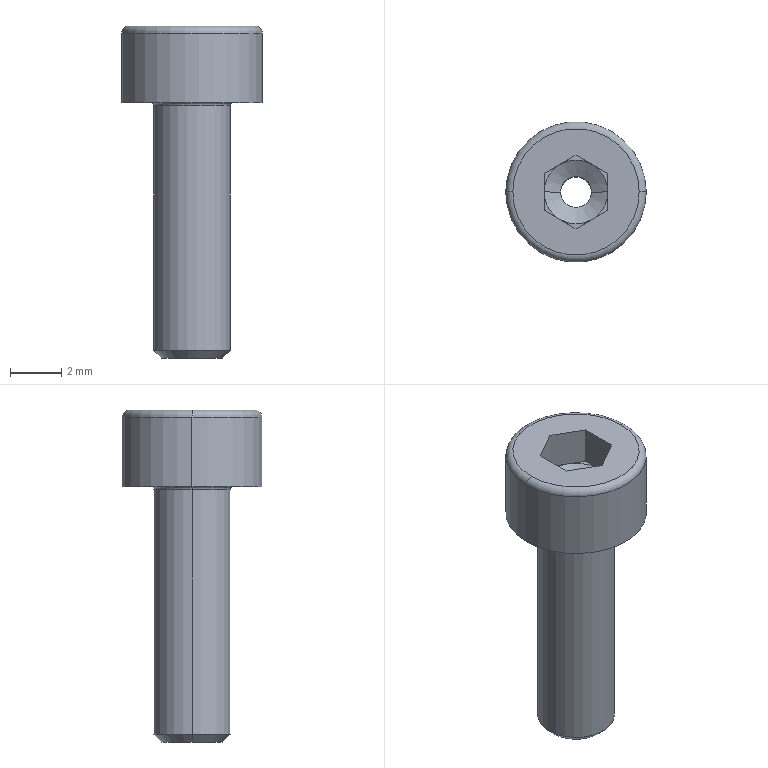Part | SolidWorks | features Fillet 2, ICE 2, Chamfer 1, Revolution 1 | 1 solid | 29 faces | box 5.5 x 5.5 x 13 mm | volume 119.572 mm3 | plane 15 | cylinder 6 | torus 4 | cone 4 | commonest cylinder face diameters 1.2 x2 3 x2 5.5 x2
STEP:
#1=CARTESIAN_POINT('',(-1.625,0.,0.));
#2=VERTEX_POINT('',#1);
#3=CARTESIAN_POINT('',(1.625,0.,0.));
#4=VERTEX_POINT('',#3);
#5=CARTESIAN_POINT('',(0.,0.,0.));
#6=DIRECTION('',(0.,0.,1.));
#7=DIRECTION('',(1.,0.,0.));
#8=AXIS2_PLACEMENT_3D('',#5,#6,#7);
#9=CIRCLE('',#8,1.625);
#10=EDGE_CURVE('',#2,#4,#9,.T.);
#11=ORIENTED_EDGE('',*,*,#10,.F.);
#12=CARTESIAN_POINT('',(-1.5,0.,-0.125));
#13=VERTEX_POINT('',#12);
#14=CARTESIAN_POINT('',(-1.625,0.,-0.125));
#15=DIRECTION('',(0.,1.,0.));
#16=DIRECTION('',(-1.,0.,0.));
#17=AXIS2_PLACEMENT_3D('',#14,#15,#16);
#18=CIRCLE('',#17,0.125);
#19=EDGE_CURVE('',#2,#13,#18,.T.);
#20=ORIENTED_EDGE('',*,*,#19,.T.);
#21=CARTESIAN_POINT('',(1.5,0.,-0.125));
#22=VERTEX_POINT('',#21);
#23=CARTESIAN_POINT('',(0.,0.,-0.125));
#24=DIRECTION('',(0.,0.,-1.));
#25=DIRECTION('',(1.,0.,0.));
#26=AXIS2_PLACEMENT_3D('',#23,#24,#25);
#27=CIRCLE('',#26,1.5);
#28=EDGE_CURVE('',#22,#13,#27,.T.);
#29=ORIENTED_EDGE('',*,*,#28,.F.);
#30=CARTESIAN_POINT('',(1.625,0.,-0.125));
#31=DIRECTION('',(0.,-1.,0.));
#32=DIRECTION('',(0.,0.,-1.));
#33=AXIS2_PLACEMENT_3D('',#30,#31,#32);
#34=CIRCLE('',#33,0.125);
#35=EDGE_CURVE('',#4,#22,#34,.T.);
#36=ORIENTED_EDGE('',*,*,#35,.F.);
#37=EDGE_LOOP('',(#11,#20,#29,#36));
#38=FACE_OUTER_BOUND('',#37,.T.);
#39=CARTESIAN_POINT('',(0.,0.,-0.125));
#40=DIRECTION('',(0.,0.,1.));
#41=DIRECTION('',(1.,0.,0.));
#42=AXIS2_PLACEMENT_3D('',#39,#40,#41);
#43=TOROIDAL_SURFACE('',#42,1.625,0.125);
#44=ADVANCED_FACE('',(#38),#43,.F.);
#45=CARTESIAN_POINT('',(-0.6,0.,1.125));
#46=VERTEX_POINT('',#45);
#47=CARTESIAN_POINT('',(0.6,0.,1.125));
#48=VERTEX_POINT('',#47);
#49=CARTESIAN_POINT('',(0.,0.,1.125));
#50=DIRECTION('',(0.,0.,1.));
#51=DIRECTION('',(1.,0.,0.));
#52=AXIS2_PLACEMENT_3D('',#49,#50,#51);
#53=CIRCLE('',#52,0.6);
#54=EDGE_CURVE('',#46,#48,#53,.T.);
#55=ORIENTED_EDGE('',*,*,#54,.F.);
#56=CARTESIAN_POINT('',(-1.25,0.,1.5));
#57=VERTEX_POINT('',#56);
#58=CARTESIAN_POINT('',(-1.25,0.,1.5));
#59=DIRECTION('',(-0.866,0.,0.5));
#60=VECTOR('',#59,1000.);
#61=LINE('',#58,#60);
#62=EDGE_CURVE('',#46,#57,#61,.T.);
#63=ORIENTED_EDGE('',*,*,#62,.T.);
#64=CARTESIAN_POINT('',(-0.625,-1.083,1.5));
#65=VERTEX_POINT('',#64);
#66=CARTESIAN_POINT('',(0.,0.,1.5));
#67=DIRECTION('',(0.,0.,1.));
#68=DIRECTION('',(1.,0.,0.));
#69=AXIS2_PLACEMENT_3D('',#66,#67,#68);
#70=CIRCLE('',#69,1.25);
#71=EDGE_CURVE('',#57,#65,#70,.T.);
#72=ORIENTED_EDGE('',*,*,#71,.T.);
#73=CARTESIAN_POINT('',(0.625,-1.083,1.5));
#74=VERTEX_POINT('',#73);
#75=CARTESIAN_POINT('',(0.,0.,1.5));
#76=DIRECTION('',(0.,0.,1.));
#77=DIRECTION('',(1.,0.,0.));
#78=AXIS2_PLACEMENT_3D('',#75,#76,#77);
#79=CIRCLE('',#78,1.25);
#80=EDGE_CURVE('',#65,#74,#79,.T.);
#81=ORIENTED_EDGE('',*,*,#80,.T.);
#82=CARTESIAN_POINT('',(1.25,0.,1.5));
#83=VERTEX_POINT('',#82);
#84=CARTESIAN_POINT('',(0.,0.,1.5));
#85=DIRECTION('',(0.,0.,1.));
#86=DIRECTION('',(1.,0.,0.));
#87=AXIS2_PLACEMENT_3D('',#84,#85,#86);
#88=CIRCLE('',#87,1.25);
#89=EDGE_CURVE('',#74,#83,#88,.T.);
#90=ORIENTED_EDGE('',*,*,#89,.T.);
#91=CARTESIAN_POINT('',(1.25,0.,1.5));
#92=DIRECTION('',(0.866,0.,0.5));
#93=VECTOR('',#92,1000.);
#94=LINE('',#91,#93);
#95=EDGE_CURVE('',#48,#83,#94,.T.);
#96=ORIENTED_EDGE('',*,*,#95,.F.);
#97=EDGE_LOOP('',(#55,#63,#72,#81,#90,#96));
#98=FACE_OUTER_BOUND('',#97,.T.);
#99=CARTESIAN_POINT('',(0.,0.,1.5));
#100=DIRECTION('',(0.,0.,1.));
#101=DIRECTION('',(1.,0.,0.));
#102=AXIS2_PLACEMENT_3D('',#99,#100,#101);
#103=CONICAL_SURFACE('',#102,1.25,1.047);
#104=ADVANCED_FACE('',(#98),#103,.F.);
#105=CARTESIAN_POINT('',(-1.2,0.,-10.));
#106=VERTEX_POINT('',#105);
#107=CARTESIAN_POINT('',(1.2,0.,-10.));
#108=VERTEX_POINT('',#107);
#109=CARTESIAN_POINT('',(0.,0.,-10.));
#110=DIRECTION('',(0.,0.,-1.));
#111=DIRECTION('',(1.,0.,0.));
#112=AXIS2_PLACEMENT_3D('',#109,#110,#111);
#113=CIRCLE('',#112,1.2);
#114=EDGE_CURVE('',#106,#108,#113,.T.);
#115=ORIENTED_EDGE('',*,*,#114,.F.);
#116=CARTESIAN_POINT('',(-1.5,0.,-9.7));
#117=VERTEX_POINT('',#116);
#118=CARTESIAN_POINT('',(-1.5,0.,-9.7));
#119=DIRECTION('',(-0.7071,0.,0.7071));
#120=VECTOR('',#119,1000.);
#121=LINE('',#118,#120);
#122=EDGE_CURVE('',#106,#117,#121,.T.);
#123=ORIENTED_EDGE('',*,*,#122,.T.);
#124=CARTESIAN_POINT('',(1.5,0.,-9.7));
#125=VERTEX_POINT('',#124);
#126=CARTESIAN_POINT('',(0.,0.,-9.7));
#127=DIRECTION('',(0.,0.,1.));
#128=DIRECTION('',(1.,0.,0.));
#129=AXIS2_PLACEMENT_3D('',#126,#127,#128);
#130=CIRCLE('',#129,1.5);
#131=EDGE_CURVE('',#125,#117,#130,.T.);
#132=ORIENTED_EDGE('',*,*,#131,.F.);
#133=CARTESIAN_POINT('',(1.5,0.,-9.7));
#134=DIRECTION('',(0.7071,0.,0.7071));
#135=VECTOR('',#134,1000.);
#136=LINE('',#133,#135);
#137=EDGE_CURVE('',#108,#125,#136,.T.);
#138=ORIENTED_EDGE('',*,*,#137,.F.);
#139=EDGE_LOOP('',(#115,#123,#132,#138));
#140=FACE_OUTER_BOUND('',#139,.T.);
#141=CARTESIAN_POINT('',(0.,0.,-9.7));
#142=DIRECTION('',(0.,0.,1.));
#143=DIRECTION('',(1.,0.,0.));
#144=AXIS2_PLACEMENT_3D('',#141,#142,#143);
#145=CONICAL_SURFACE('',#144,1.5,0.7854);
#146=ADVANCED_FACE('',(#140),#145,.T.);
#147=CARTESIAN_POINT('',(2.475,0.,3.));
#148=VERTEX_POINT('',#147);
#149=CARTESIAN_POINT('',(-2.475,0.,3.));
#150=VERTEX_POINT('',#149);
#151=CARTESIAN_POINT('',(0.,0.,3.));
#152=DIRECTION('',(0.,0.,1.));
#153=DIRECTION('',(-1.,0.,0.));
#154=AXIS2_PLACEMENT_3D('',#151,#152,#153);
#155=CIRCLE('',#154,2.475);
#156=EDGE_CURVE('',#148,#150,#155,.T.);
#157=ORIENTED_EDGE('',*,*,#156,.F.);
#158=CARTESIAN_POINT('',(2.75,0.,2.725));
#159=VERTEX_POINT('',#158);
#160=CARTESIAN_POINT('',(2.475,0.,2.725));
#161=DIRECTION('',(0.,1.,0.));
#162=DIRECTION('',(-1.,0.,0.));
#163=AXIS2_PLACEMENT_3D('',#160,#161,#162);
#164=CIRCLE('',#163,0.275);
#165=EDGE_CURVE('',#148,#159,#164,.T.);
#166=ORIENTED_EDGE('',*,*,#165,.T.);
#167=CARTESIAN_POINT('',(-2.75,0.,2.725));
#168=VERTEX_POINT('',#167);
#169=CARTESIAN_POINT('',(0.,0.,2.725));
#170=DIRECTION('',(0.,0.,-1.));
#171=DIRECTION('',(-1.,0.,0.));
#172=AXIS2_PLACEMENT_3D('',#169,#170,#171);
#173=CIRCLE('',#172,2.75);
#174=EDGE_CURVE('',#168,#159,#173,.T.);
#175=ORIENTED_EDGE('',*,*,#174,.F.);
#176=CARTESIAN_POINT('',(-2.475,0.,2.725));
#177=DIRECTION('',(0.,-1.,0.));
#178=DIRECTION('',(0.,0.,-1.));
#179=AXIS2_PLACEMENT_3D('',#176,#177,#178);
#180=CIRCLE('',#179,0.275);
#181=EDGE_CURVE('',#150,#168,#180,.T.);
#182=ORIENTED_EDGE('',*,*,#181,.F.);
#183=EDGE_LOOP('',(#157,#166,#175,#182));
#184=FACE_OUTER_BOUND('',#183,.T.);
#185=CARTESIAN_POINT('',(0.,0.,2.725));
#186=DIRECTION('',(0.,0.,-1.));
#187=DIRECTION('',(-1.,0.,0.));
#188=AXIS2_PLACEMENT_3D('',#185,#186,#187);
#189=TOROIDAL_SURFACE('',#188,2.475,0.275);
#190=ADVANCED_FACE('',(#184),#189,.T.);
#191=ORIENTED_EDGE('',*,*,#131,.T.);
#192=CARTESIAN_POINT('',(-1.5,0.,3.));
#193=DIRECTION('',(0.,0.,1.));
#194=VECTOR('',#193,1000.);
#195=LINE('',#192,#194);
#196=EDGE_CURVE('',#117,#13,#195,.T.);
#197=ORIENTED_EDGE('',*,*,#196,.T.);
#198=CARTESIAN_POINT('',(0.,0.,-0.125));
#199=DIRECTION('',(0.,0.,-1.));
#200=DIRECTION('',(1.,0.,0.));
#201=AXIS2_PLACEMENT_3D('',#198,#199,#200);
#202=CIRCLE('',#201,1.5);
#203=EDGE_CURVE('',#13,#22,#202,.T.);
#204=ORIENTED_EDGE('',*,*,#203,.T.);
#205=CARTESIAN_POINT('',(1.5,0.,3.));
#206=DIRECTION('',(0.,0.,1.));
#207=VECTOR('',#206,1000.);
#208=LINE('',#205,#207);
#209=EDGE_CURVE('',#125,#22,#208,.T.);
#210=ORIENTED_EDGE('',*,*,#209,.F.);
#211=EDGE_LOOP('',(#191,#197,#204,#210));
#212=FACE_OUTER_BOUND('',#211,.T.);
#213=CARTESIAN_POINT('',(0.,0.,3.));
#214=DIRECTION('',(0.,0.,1.));
#215=DIRECTION('',(1.,0.,0.));
#216=AXIS2_PLACEMENT_3D('',#213,#214,#215);
#217=CYLINDRICAL_SURFACE('',#216,1.5);
#218=ADVANCED_FACE('',(#212),#217,.T.);
#219=CARTESIAN_POINT('',(2.75,0.,0.));
#220=VERTEX_POINT('',#219);
#221=CARTESIAN_POINT('',(-2.75,0.,0.));
#222=VERTEX_POINT('',#221);
#223=CARTESIAN_POINT('',(0.,0.,0.));
#224=DIRECTION('',(0.,0.,1.));
#225=DIRECTION('',(1.,0.,0.));
#226=AXIS2_PLACEMENT_3D('',#223,#224,#225);
#227=CIRCLE('',#226,2.75);
#228=EDGE_CURVE('',#220,#222,#227,.T.);
#229=ORIENTED_EDGE('',*,*,#228,.T.);
#230=CARTESIAN_POINT('',(-2.75,0.,3.));
#231=DIRECTION('',(0.,0.,1.));
#232=VECTOR('',#231,1000.);
#233=LINE('',#230,#232);
#234=EDGE_CURVE('',#222,#168,#233,.T.);
#235=ORIENTED_EDGE('',*,*,#234,.T.);
#236=ORIENTED_EDGE('',*,*,#174,.T.);
#237=CARTESIAN_POINT('',(2.75,0.,3.));
#238=DIRECTION('',(0.,0.,1.));
#239=VECTOR('',#238,1000.);
#240=LINE('',#237,#239);
#241=EDGE_CURVE('',#220,#159,#240,.T.);
#242=ORIENTED_EDGE('',*,*,#241,.F.);
#243=EDGE_LOOP('',(#229,#235,#236,#242));
#244=FACE_OUTER_BOUND('',#243,.T.);
#245=CARTESIAN_POINT('',(0.,0.,3.));
#246=DIRECTION('',(0.,0.,1.));
#247=DIRECTION('',(1.,0.,0.));
#248=AXIS2_PLACEMENT_3D('',#245,#246,#247);
#249=CYLINDRICAL_SURFACE('',#248,2.75);
#250=ADVANCED_FACE('',(#244),#249,.T.);
#251=CARTESIAN_POINT('',(-0.6,0.,-10.));
#252=VERTEX_POINT('',#251);
#253=CARTESIAN_POINT('',(0.6,0.,-10.));
#254=VERTEX_POINT('',#253);
#255=CARTESIAN_POINT('',(0.,0.,-10.));
#256=DIRECTION('',(0.,0.,1.));
#257=DIRECTION('',(1.,0.,0.));
#258=AXIS2_PLACEMENT_3D('',#255,#256,#257);
#259=CIRCLE('',#258,0.6);
#260=EDGE_CURVE('',#252,#254,#259,.T.);
#261=ORIENTED_EDGE('',*,*,#260,.F.);
#262=CARTESIAN_POINT('',(-0.6,0.,3.));
#263=DIRECTION('',(0.,0.,1.));
#264=VECTOR('',#263,1000.);
#265=LINE('',#262,#264);
#266=EDGE_CURVE('',#252,#46,#265,.T.);
#267=ORIENTED_EDGE('',*,*,#266,.T.);
#268=ORIENTED_EDGE('',*,*,#54,.T.);
#269=CARTESIAN_POINT('',(0.6,0.,3.));
#270=DIRECTION('',(0.,0.,1.));
#271=VECTOR('',#270,1000.);
#272=LINE('',#269,#271);
#273=EDGE_CURVE('',#254,#48,#272,.T.);
#274=ORIENTED_EDGE('',*,*,#273,.F.);
#275=EDGE_LOOP('',(#261,#267,#268,#274));
#276=FACE_OUTER_BOUND('',#275,.T.);
#277=CARTESIAN_POINT('',(0.,0.,3.));
#278=DIRECTION('',(0.,0.,1.));
#279=DIRECTION('',(1.,0.,0.));
#280=AXIS2_PLACEMENT_3D('',#277,#278,#279);
#281=CYLINDRICAL_SURFACE('',#280,0.6);
#282=ADVANCED_FACE('',(#276),#281,.F.);
#283=CARTESIAN_POINT('',(0.625,1.083,1.5));
#284=VERTEX_POINT('',#283);
#285=CARTESIAN_POINT('',(0.,0.,1.5));
#286=DIRECTION('',(0.,0.,1.));
#287=DIRECTION('',(1.,0.,0.));
#288=AXIS2_PLACEMENT_3D('',#285,#286,#287);
#289=CIRCLE('',#288,1.25);
#290=EDGE_CURVE('',#83,#284,#289,.T.);
#291=ORIENTED_EDGE('',*,*,#290,.F.);
#292=CARTESIAN_POINT('',(1.25,0.7217,1.5));
#293=VERTEX_POINT('',#292);
#294=CARTESIAN_POINT('',(1.25,-0.7217,1.5));
#295=DIRECTION('',(0.,1.,0.));
#296=VECTOR('',#295,1000.);
#297=LINE('',#294,#296);
#298=EDGE_CURVE('',#83,#293,#297,.T.);
#299=ORIENTED_EDGE('',*,*,#298,.T.);
#300=CARTESIAN_POINT('',(1.25,0.7217,1.5));
#301=DIRECTION('',(-0.866,0.5,0.));
#302=VECTOR('',#301,1000.);
#303=LINE('',#300,#302);
#304=EDGE_CURVE('',#293,#284,#303,.T.);
#305=ORIENTED_EDGE('',*,*,#304,.T.);
#306=EDGE_LOOP('',(#291,#299,#305));
#307=FACE_OUTER_BOUND('',#306,.T.);
#308=CARTESIAN_POINT('',(0.,1.443,1.5));
#309=DIRECTION('',(0.,0.,1.));
#310=DIRECTION('',(1.,0.,0.));
#311=AXIS2_PLACEMENT_3D('',#308,#309,#310);
#312=PLANE('',#311);
#313=ADVANCED_FACE('',(#307),#312,.T.);
#314=CARTESIAN_POINT('',(-0.625,1.083,1.5));
#315=VERTEX_POINT('',#314);
#316=CARTESIAN_POINT('',(0.,0.,1.5));
#317=DIRECTION('',(0.,0.,1.));
#318=DIRECTION('',(1.,0.,0.));
#319=AXIS2_PLACEMENT_3D('',#316,#317,#318);
#320=CIRCLE('',#319,1.25);
#321=EDGE_CURVE('',#284,#315,#320,.T.);
#322=ORIENTED_EDGE('',*,*,#321,.F.);
#323=CARTESIAN_POINT('',(0.,1.443,1.5));
#324=VERTEX_POINT('',#323);
#325=CARTESIAN_POINT('',(1.25,0.7217,1.5));
#326=DIRECTION('',(-0.866,0.5,0.));
#327=VECTOR('',#326,1000.);
#328=LINE('',#325,#327);
#329=EDGE_CURVE('',#284,#324,#328,.T.);
#330=ORIENTED_EDGE('',*,*,#329,.T.);
#331=CARTESIAN_POINT('',(0.,1.443,1.5));
#332=DIRECTION('',(-0.866,-0.5,0.));
#333=VECTOR('',#332,1000.);
#334=LINE('',#331,#333);
#335=EDGE_CURVE('',#324,#315,#334,.T.);
#336=ORIENTED_EDGE('',*,*,#335,.T.);
#337=EDGE_LOOP('',(#322,#330,#336));
#338=FACE_OUTER_BOUND('',#337,.T.);
#339=CARTESIAN_POINT('',(0.,1.443,1.5));
#340=DIRECTION('',(0.,0.,1.));
#341=DIRECTION('',(1.,0.,0.));
#342=AXIS2_PLACEMENT_3D('',#339,#340,#341);
#343=PLANE('',#342);
#344=ADVANCED_FACE('',(#338),#343,.T.);
#345=CARTESIAN_POINT('',(0.,0.,1.5));
#346=DIRECTION('',(0.,0.,1.));
#347=DIRECTION('',(1.,0.,0.));
#348=AXIS2_PLACEMENT_3D('',#345,#346,#347);
#349=CIRCLE('',#348,1.25);
#350=EDGE_CURVE('',#315,#57,#349,.T.);
#351=ORIENTED_EDGE('',*,*,#350,.F.);
#352=CARTESIAN_POINT('',(-1.25,0.7217,1.5));
#353=VERTEX_POINT('',#352);
#354=CARTESIAN_POINT('',(0.,1.443,1.5));
#355=DIRECTION('',(-0.866,-0.5,0.));
#356=VECTOR('',#355,1000.);
#357=LINE('',#354,#356);
#358=EDGE_CURVE('',#315,#353,#357,.T.);
#359=ORIENTED_EDGE('',*,*,#358,.T.);
#360=CARTESIAN_POINT('',(-1.25,0.7217,1.5));
#361=DIRECTION('',(0.,-1.,0.));
#362=VECTOR('',#361,1000.);
#363=LINE('',#360,#362);
#364=EDGE_CURVE('',#353,#57,#363,.T.);
#365=ORIENTED_EDGE('',*,*,#364,.T.);
#366=EDGE_LOOP('',(#351,#359,#365));
#367=FACE_OUTER_BOUND('',#366,.T.);
#368=CARTESIAN_POINT('',(0.,1.443,1.5));
#369=DIRECTION('',(0.,0.,1.));
#370=DIRECTION('',(1.,0.,0.));
#371=AXIS2_PLACEMENT_3D('',#368,#369,#370);
#372=PLANE('',#371);
#373=ADVANCED_FACE('',(#367),#372,.T.);
#374=ORIENTED_EDGE('',*,*,#71,.F.);
#375=CARTESIAN_POINT('',(-1.25,-0.7217,1.5));
#376=VERTEX_POINT('',#375);
#377=CARTESIAN_POINT('',(-1.25,0.7217,1.5));
#378=DIRECTION('',(0.,-1.,0.));
#379=VECTOR('',#378,1000.);
#380=LINE('',#377,#379);
#381=EDGE_CURVE('',#57,#376,#380,.T.);
#382=ORIENTED_EDGE('',*,*,#381,.T.);
#383=CARTESIAN_POINT('',(-1.25,-0.7217,1.5));
#384=DIRECTION('',(0.866,-0.5,0.));
#385=VECTOR('',#384,1000.);
#386=LINE('',#383,#385);
#387=EDGE_CURVE('',#376,#65,#386,.T.);
#388=ORIENTED_EDGE('',*,*,#387,.T.);
#389=EDGE_LOOP('',(#374,#382,#388));
#390=FACE_OUTER_BOUND('',#389,.T.);
#391=CARTESIAN_POINT('',(0.,1.443,1.5));
#392=DIRECTION('',(0.,0.,1.));
#393=DIRECTION('',(1.,0.,0.));
#394=AXIS2_PLACEMENT_3D('',#391,#392,#393);
#395=PLANE('',#394);
#396=ADVANCED_FACE('',(#390),#395,.T.);
#397=ORIENTED_EDGE('',*,*,#80,.F.);
#398=CARTESIAN_POINT('',(0.,-1.443,1.5));
#399=VERTEX_POINT('',#398);
#400=CARTESIAN_POINT('',(-1.25,-0.7217,1.5));
#401=DIRECTION('',(0.866,-0.5,0.));
#402=VECTOR('',#401,1000.);
#403=LINE('',#400,#402);
#404=EDGE_CURVE('',#65,#399,#403,.T.);
#405=ORIENTED_EDGE('',*,*,#404,.T.);
#406=CARTESIAN_POINT('',(0.,-1.443,1.5));
#407=DIRECTION('',(0.866,0.5,0.));
#408=VECTOR('',#407,1000.);
#409=LINE('',#406,#408);
#410=EDGE_CURVE('',#399,#74,#409,.T.);
#411=ORIENTED_EDGE('',*,*,#410,.T.);
#412=EDGE_LOOP('',(#397,#405,#411));
#413=FACE_OUTER_BOUND('',#412,.T.);
#414=CARTESIAN_POINT('',(0.,1.443,1.5));
#415=DIRECTION('',(0.,0.,1.));
#416=DIRECTION('',(1.,0.,0.));
#417=AXIS2_PLACEMENT_3D('',#414,#415,#416);
#418=PLANE('',#417);
#419=ADVANCED_FACE('',(#413),#418,.T.);
#420=ORIENTED_EDGE('',*,*,#266,.F.);
#421=CARTESIAN_POINT('',(0.,0.,-10.));
#422=DIRECTION('',(0.,0.,1.));
#423=DIRECTION('',(1.,0.,0.));
#424=AXIS2_PLACEMENT_3D('',#421,#422,#423);
#425=CIRCLE('',#424,0.6);
#426=EDGE_CURVE('',#254,#252,#425,.T.);
#427=ORIENTED_EDGE('',*,*,#426,.F.);
#428=ORIENTED_EDGE('',*,*,#273,.T.);
#429=CARTESIAN_POINT('',(0.,0.,1.125));
#430=DIRECTION('',(0.,0.,1.));
#431=DIRECTION('',(1.,0.,0.));
#432=AXIS2_PLACEMENT_3D('',#429,#430,#431);
#433=CIRCLE('',#432,0.6);
#434=EDGE_CURVE('',#48,#46,#433,.T.);
#435=ORIENTED_EDGE('',*,*,#434,.T.);
#436=EDGE_LOOP('',(#420,#427,#428,#435));
#437=FACE_OUTER_BOUND('',#436,.T.);
#438=CARTESIAN_POINT('',(0.,0.,3.));
#439=DIRECTION('',(0.,0.,1.));
#440=DIRECTION('',(1.,0.,0.));
#441=AXIS2_PLACEMENT_3D('',#438,#439,#440);
#442=CYLINDRICAL_SURFACE('',#441,0.6);
#443=ADVANCED_FACE('',(#437),#442,.F.);
#444=ORIENTED_EDGE('',*,*,#234,.F.);
#445=CARTESIAN_POINT('',(0.,0.,0.));
#446=DIRECTION('',(0.,0.,1.));
#447=DIRECTION('',(1.,0.,0.));
#448=AXIS2_PLACEMENT_3D('',#445,#446,#447);
#449=CIRCLE('',#448,2.75);
#450=EDGE_CURVE('',#222,#220,#449,.T.);
#451=ORIENTED_EDGE('',*,*,#450,.T.);
#452=ORIENTED_EDGE('',*,*,#241,.T.);
#453=CARTESIAN_POINT('',(0.,0.,2.725));
#454=DIRECTION('',(0.,0.,-1.));
#455=DIRECTION('',(-1.,0.,0.));
#456=AXIS2_PLACEMENT_3D('',#453,#454,#455);
#457=CIRCLE('',#456,2.75);
#458=EDGE_CURVE('',#159,#168,#457,.T.);
#459=ORIENTED_EDGE('',*,*,#458,.T.);
#460=EDGE_LOOP('',(#444,#451,#452,#459));
#461=FACE_OUTER_BOUND('',#460,.T.);
#462=CARTESIAN_POINT('',(0.,0.,3.));
#463=DIRECTION('',(0.,0.,1.));
#464=DIRECTION('',(1.,0.,0.));
#465=AXIS2_PLACEMENT_3D('',#462,#463,#464);
#466=CYLINDRICAL_SURFACE('',#465,2.75);
#467=ADVANCED_FACE('',(#461),#466,.T.);
#468=CARTESIAN_POINT('',(0.,0.,0.));
#469=DIRECTION('',(0.,0.,1.));
#470=DIRECTION('',(1.,0.,0.));
#471=AXIS2_PLACEMENT_3D('',#468,#469,#470);
#472=CIRCLE('',#471,1.625);
#473=EDGE_CURVE('',#4,#2,#472,.T.);
#474=ORIENTED_EDGE('',*,*,#473,.T.);
#475=ORIENTED_EDGE('',*,*,#10,.T.);
#476=EDGE_LOOP('',(#474,#475));
#477=FACE_BOUND('',#476,.T.);
#478=ORIENTED_EDGE('',*,*,#228,.F.);
#479=ORIENTED_EDGE('',*,*,#450,.F.);
#480=EDGE_LOOP('',(#478,#479));
#481=FACE_OUTER_BOUND('',#480,.T.);
#482=CARTESIAN_POINT('',(0.,2.75,0.));
#483=DIRECTION('',(0.,0.,1.));
#484=DIRECTION('',(1.,0.,0.));
#485=AXIS2_PLACEMENT_3D('',#482,#483,#484);
#486=PLANE('',#485);
#487=ADVANCED_FACE('',(#477,#481),#486,.F.);
#488=ORIENTED_EDGE('',*,*,#196,.F.);
#489=CARTESIAN_POINT('',(0.,0.,-9.7));
#490=DIRECTION('',(0.,0.,1.));
#491=DIRECTION('',(1.,0.,0.));
#492=AXIS2_PLACEMENT_3D('',#489,#490,#491);
#493=CIRCLE('',#492,1.5);
#494=EDGE_CURVE('',#117,#125,#493,.T.);
#495=ORIENTED_EDGE('',*,*,#494,.T.);
#496=ORIENTED_EDGE('',*,*,#209,.T.);
#497=ORIENTED_EDGE('',*,*,#28,.T.);
#498=EDGE_LOOP('',(#488,#495,#496,#497));
#499=FACE_OUTER_BOUND('',#498,.T.);
#500=CARTESIAN_POINT('',(0.,0.,3.));
#501=DIRECTION('',(0.,0.,1.));
#502=DIRECTION('',(1.,0.,0.));
#503=AXIS2_PLACEMENT_3D('',#500,#501,#502);
#504=CYLINDRICAL_SURFACE('',#503,1.5);
#505=ADVANCED_FACE('',(#499),#504,.T.);
#506=CARTESIAN_POINT('',(0.,0.,-10.));
#507=DIRECTION('',(0.,0.,-1.));
#508=DIRECTION('',(1.,0.,0.));
#509=AXIS2_PLACEMENT_3D('',#506,#507,#508);
#510=CIRCLE('',#509,1.2);
#511=EDGE_CURVE('',#108,#106,#510,.T.);
#512=ORIENTED_EDGE('',*,*,#511,.T.);
#513=ORIENTED_EDGE('',*,*,#114,.T.);
#514=EDGE_LOOP('',(#512,#513));
#515=FACE_OUTER_BOUND('',#514,.T.);
#516=ORIENTED_EDGE('',*,*,#426,.T.);
#517=ORIENTED_EDGE('',*,*,#260,.T.);
#518=EDGE_LOOP('',(#516,#517));
#519=FACE_BOUND('',#518,.T.);
#520=CARTESIAN_POINT('',(0.,1.5,-10.));
#521=DIRECTION('',(0.,0.,1.));
#522=DIRECTION('',(1.,0.,0.));
#523=AXIS2_PLACEMENT_3D('',#520,#521,#522);
#524=PLANE('',#523);
#525=ADVANCED_FACE('',(#515,#519),#524,.F.);
#526=CARTESIAN_POINT('',(0.,0.,3.));
#527=DIRECTION('',(0.,0.,1.));
#528=DIRECTION('',(-1.,0.,0.));
#529=AXIS2_PLACEMENT_3D('',#526,#527,#528);
#530=CIRCLE('',#529,2.475);
#531=EDGE_CURVE('',#150,#148,#530,.T.);
#532=ORIENTED_EDGE('',*,*,#531,.T.);
#533=ORIENTED_EDGE('',*,*,#156,.T.);
#534=EDGE_LOOP('',(#532,#533));
#535=FACE_OUTER_BOUND('',#534,.T.);
#536=CARTESIAN_POINT('',(0.,1.443,3.));
#537=VERTEX_POINT('',#536);
#538=CARTESIAN_POINT('',(-1.25,0.7217,3.));
#539=VERTEX_POINT('',#538);
#540=CARTESIAN_POINT('',(0.,1.443,3.));
#541=DIRECTION('',(-0.866,-0.5,0.));
#542=VECTOR('',#541,1000.);
#543=LINE('',#540,#542);
#544=EDGE_CURVE('',#537,#539,#543,.T.);
#545=ORIENTED_EDGE('',*,*,#544,.F.);
#546=CARTESIAN_POINT('',(1.25,0.7217,3.));
#547=VERTEX_POINT('',#546);
#548=CARTESIAN_POINT('',(1.25,0.7217,3.));
#549=DIRECTION('',(-0.866,0.5,0.));
#550=VECTOR('',#549,1000.);
#551=LINE('',#548,#550);
#552=EDGE_CURVE('',#547,#537,#551,.T.);
#553=ORIENTED_EDGE('',*,*,#552,.F.);
#554=CARTESIAN_POINT('',(1.25,-0.7217,3.));
#555=VERTEX_POINT('',#554);
#556=CARTESIAN_POINT('',(1.25,-0.7217,3.));
#557=DIRECTION('',(0.,1.,0.));
#558=VECTOR('',#557,1000.);
#559=LINE('',#556,#558);
#560=EDGE_CURVE('',#555,#547,#559,.T.);
#561=ORIENTED_EDGE('',*,*,#560,.F.);
#562=CARTESIAN_POINT('',(0.,-1.443,3.));
#563=VERTEX_POINT('',#562);
#564=CARTESIAN_POINT('',(0.,-1.443,3.));
#565=DIRECTION('',(0.866,0.5,0.));
#566=VECTOR('',#565,1000.);
#567=LINE('',#564,#566);
#568=EDGE_CURVE('',#563,#555,#567,.T.);
#569=ORIENTED_EDGE('',*,*,#568,.F.);
#570=CARTESIAN_POINT('',(-1.25,-0.7217,3.));
#571=VERTEX_POINT('',#570);
#572=CARTESIAN_POINT('',(-1.25,-0.7217,3.));
#573=DIRECTION('',(0.866,-0.5,0.));
#574=VECTOR('',#573,1000.);
#575=LINE('',#572,#574);
#576=EDGE_CURVE('',#571,#563,#575,.T.);
#577=ORIENTED_EDGE('',*,*,#576,.F.);
#578=CARTESIAN_POINT('',(-1.25,0.7217,3.));
#579=DIRECTION('',(0.,-1.,0.));
#580=VECTOR('',#579,1000.);
#581=LINE('',#578,#580);
#582=EDGE_CURVE('',#539,#571,#581,.T.);
#583=ORIENTED_EDGE('',*,*,#582,.F.);
#584=EDGE_LOOP('',(#545,#553,#561,#569,#577,#583));
#585=FACE_BOUND('',#584,.T.);
#586=CARTESIAN_POINT('',(0.,0.6,3.));
#587=DIRECTION('',(0.,0.,-1.));
#588=DIRECTION('',(-1.,0.,0.));
#589=AXIS2_PLACEMENT_3D('',#586,#587,#588);
#590=PLANE('',#589);
#591=ADVANCED_FACE('',(#535,#585),#590,.F.);
#592=ORIENTED_EDGE('',*,*,#89,.F.);
#593=CARTESIAN_POINT('',(1.25,-0.7217,1.5));
#594=VERTEX_POINT('',#593);
#595=CARTESIAN_POINT('',(0.,-1.443,1.5));
#596=DIRECTION('',(0.866,0.5,0.));
#597=VECTOR('',#596,1000.);
#598=LINE('',#595,#597);
#599=EDGE_CURVE('',#74,#594,#598,.T.);
#600=ORIENTED_EDGE('',*,*,#599,.T.);
#601=CARTESIAN_POINT('',(1.25,-0.7217,1.5));
#602=DIRECTION('',(0.,1.,0.));
#603=VECTOR('',#602,1000.);
#604=LINE('',#601,#603);
#605=EDGE_CURVE('',#594,#83,#604,.T.);
#606=ORIENTED_EDGE('',*,*,#605,.T.);
#607=EDGE_LOOP('',(#592,#600,#606));
#608=FACE_OUTER_BOUND('',#607,.T.);
#609=CARTESIAN_POINT('',(0.,1.443,1.5));
#610=DIRECTION('',(0.,0.,1.));
#611=DIRECTION('',(1.,0.,0.));
#612=AXIS2_PLACEMENT_3D('',#609,#610,#611);
#613=PLANE('',#612);
#614=ADVANCED_FACE('',(#608),#613,.T.);
#615=ORIENTED_EDGE('',*,*,#552,.T.);
#616=CARTESIAN_POINT('',(0.,1.443,1.5));
#617=DIRECTION('',(0.,0.,1.));
#618=VECTOR('',#617,1000.);
#619=LINE('',#616,#618);
#620=EDGE_CURVE('',#324,#537,#619,.T.);
#621=ORIENTED_EDGE('',*,*,#620,.F.);
#622=ORIENTED_EDGE('',*,*,#329,.F.);
#623=ORIENTED_EDGE('',*,*,#304,.F.);
#624=CARTESIAN_POINT('',(1.25,0.7217,1.5));
#625=DIRECTION('',(0.,0.,1.));
#626=VECTOR('',#625,1000.);
#627=LINE('',#624,#626);
#628=EDGE_CURVE('',#293,#547,#627,.T.);
#629=ORIENTED_EDGE('',*,*,#628,.T.);
#630=EDGE_LOOP('',(#615,#621,#622,#623,#629));
#631=FACE_OUTER_BOUND('',#630,.T.);
#632=CARTESIAN_POINT('',(1.25,0.7217,1.5));
#633=DIRECTION('',(0.5,0.866,0.));
#634=DIRECTION('',(-0.866,0.5,0.));
#635=AXIS2_PLACEMENT_3D('',#632,#633,#634);
#636=PLANE('',#635);
#637=ADVANCED_FACE('',(#631),#636,.F.);
#638=ORIENTED_EDGE('',*,*,#560,.T.);
#639=ORIENTED_EDGE('',*,*,#628,.F.);
#640=ORIENTED_EDGE('',*,*,#298,.F.);
#641=ORIENTED_EDGE('',*,*,#605,.F.);
#642=CARTESIAN_POINT('',(1.25,-0.7217,1.5));
#643=DIRECTION('',(0.,0.,1.));
#644=VECTOR('',#643,1000.);
#645=LINE('',#642,#644);
#646=EDGE_CURVE('',#594,#555,#645,.T.);
#647=ORIENTED_EDGE('',*,*,#646,.T.);
#648=EDGE_LOOP('',(#638,#639,#640,#641,#647));
#649=FACE_OUTER_BOUND('',#648,.T.);
#650=CARTESIAN_POINT('',(1.25,-0.7217,1.5));
#651=DIRECTION('',(1.,0.,0.));
#652=DIRECTION('',(0.,0.,-1.));
#653=AXIS2_PLACEMENT_3D('',#650,#651,#652);
#654=PLANE('',#653);
#655=ADVANCED_FACE('',(#649),#654,.F.);
#656=ORIENTED_EDGE('',*,*,#568,.T.);
#657=ORIENTED_EDGE('',*,*,#646,.F.);
#658=ORIENTED_EDGE('',*,*,#599,.F.);
#659=ORIENTED_EDGE('',*,*,#410,.F.);
#660=CARTESIAN_POINT('',(0.,-1.443,1.5));
#661=DIRECTION('',(0.,0.,1.));
#662=VECTOR('',#661,1000.);
#663=LINE('',#660,#662);
#664=EDGE_CURVE('',#399,#563,#663,.T.);
#665=ORIENTED_EDGE('',*,*,#664,.T.);
#666=EDGE_LOOP('',(#656,#657,#658,#659,#665));
#667=FACE_OUTER_BOUND('',#666,.T.);
#668=CARTESIAN_POINT('',(0.,-1.443,1.5));
#669=DIRECTION('',(0.5,-0.866,0.));
#670=DIRECTION('',(0.866,0.5,0.));
#671=AXIS2_PLACEMENT_3D('',#668,#669,#670);
#672=PLANE('',#671);
#673=ADVANCED_FACE('',(#667),#672,.F.);
#674=ORIENTED_EDGE('',*,*,#576,.T.);
#675=ORIENTED_EDGE('',*,*,#664,.F.);
#676=ORIENTED_EDGE('',*,*,#404,.F.);
#677=ORIENTED_EDGE('',*,*,#387,.F.);
#678=CARTESIAN_POINT('',(-1.25,-0.7217,1.5));
#679=DIRECTION('',(0.,0.,1.));
#680=VECTOR('',#679,1000.);
#681=LINE('',#678,#680);
#682=EDGE_CURVE('',#376,#571,#681,.T.);
#683=ORIENTED_EDGE('',*,*,#682,.T.);
#684=EDGE_LOOP('',(#674,#675,#676,#677,#683));
#685=FACE_OUTER_BOUND('',#684,.T.);
#686=CARTESIAN_POINT('',(-1.25,-0.7217,1.5));
#687=DIRECTION('',(-0.5,-0.866,0.));
#688=DIRECTION('',(0.866,-0.5,0.));
#689=AXIS2_PLACEMENT_3D('',#686,#687,#688);
#690=PLANE('',#689);
#691=ADVANCED_FACE('',(#685),#690,.F.);
#692=ORIENTED_EDGE('',*,*,#582,.T.);
#693=ORIENTED_EDGE('',*,*,#682,.F.);
#694=ORIENTED_EDGE('',*,*,#381,.F.);
#695=ORIENTED_EDGE('',*,*,#364,.F.);
#696=CARTESIAN_POINT('',(-1.25,0.7217,1.5));
#697=DIRECTION('',(0.,0.,1.));
#698=VECTOR('',#697,1000.);
#699=LINE('',#696,#698);
#700=EDGE_CURVE('',#353,#539,#699,.T.);
#701=ORIENTED_EDGE('',*,*,#700,.T.);
#702=EDGE_LOOP('',(#692,#693,#694,#695,#701));
#703=FACE_OUTER_BOUND('',#702,.T.);
#704=CARTESIAN_POINT('',(-1.25,0.7217,1.5));
#705=DIRECTION('',(-1.,0.,0.));
#706=DIRECTION('',(0.,-1.,0.));
#707=AXIS2_PLACEMENT_3D('',#704,#705,#706);
#708=PLANE('',#707);
#709=ADVANCED_FACE('',(#703),#708,.F.);
#710=ORIENTED_EDGE('',*,*,#544,.T.);
#711=ORIENTED_EDGE('',*,*,#700,.F.);
#712=ORIENTED_EDGE('',*,*,#358,.F.);
#713=ORIENTED_EDGE('',*,*,#335,.F.);
#714=ORIENTED_EDGE('',*,*,#620,.T.);
#715=EDGE_LOOP('',(#710,#711,#712,#713,#714));
#716=FACE_OUTER_BOUND('',#715,.T.);
#717=CARTESIAN_POINT('',(0.,1.443,1.5));
#718=DIRECTION('',(-0.5,0.866,0.));
#719=DIRECTION('',(-0.866,-0.5,0.));
#720=AXIS2_PLACEMENT_3D('',#717,#718,#719);
#721=PLANE('',#720);
#722=ADVANCED_FACE('',(#716),#721,.F.);
#723=ORIENTED_EDGE('',*,*,#165,.F.);
#724=ORIENTED_EDGE('',*,*,#531,.F.);
#725=ORIENTED_EDGE('',*,*,#181,.T.);
#726=ORIENTED_EDGE('',*,*,#458,.F.);
#727=EDGE_LOOP('',(#723,#724,#725,#726));
#728=FACE_OUTER_BOUND('',#727,.T.);
#729=CARTESIAN_POINT('',(0.,0.,2.725));
#730=DIRECTION('',(0.,0.,-1.));
#731=DIRECTION('',(-1.,0.,0.));
#732=AXIS2_PLACEMENT_3D('',#729,#730,#731);
#733=TOROIDAL_SURFACE('',#732,2.475,0.275);
#734=ADVANCED_FACE('',(#728),#733,.T.);
#735=ORIENTED_EDGE('',*,*,#122,.F.);
#736=ORIENTED_EDGE('',*,*,#511,.F.);
#737=ORIENTED_EDGE('',*,*,#137,.T.);
#738=ORIENTED_EDGE('',*,*,#494,.F.);
#739=EDGE_LOOP('',(#735,#736,#737,#738));
#740=FACE_OUTER_BOUND('',#739,.T.);
#741=CARTESIAN_POINT('',(0.,0.,-9.7));
#742=DIRECTION('',(0.,0.,1.));
#743=DIRECTION('',(1.,0.,0.));
#744=AXIS2_PLACEMENT_3D('',#741,#742,#743);
#745=CONICAL_SURFACE('',#744,1.5,0.7854);
#746=ADVANCED_FACE('',(#740),#745,.T.);
#747=ORIENTED_EDGE('',*,*,#62,.F.);
#748=ORIENTED_EDGE('',*,*,#434,.F.);
#749=ORIENTED_EDGE('',*,*,#95,.T.);
#750=ORIENTED_EDGE('',*,*,#290,.T.);
#751=ORIENTED_EDGE('',*,*,#321,.T.);
#752=ORIENTED_EDGE('',*,*,#350,.T.);
#753=EDGE_LOOP('',(#747,#748,#749,#750,#751,#752));
#754=FACE_OUTER_BOUND('',#753,.T.);
#755=CARTESIAN_POINT('',(0.,0.,1.5));
#756=DIRECTION('',(0.,0.,1.));
#757=DIRECTION('',(1.,0.,0.));
#758=AXIS2_PLACEMENT_3D('',#755,#756,#757);
#759=CONICAL_SURFACE('',#758,1.25,1.047);
#760=ADVANCED_FACE('',(#754),#759,.F.);
#761=ORIENTED_EDGE('',*,*,#19,.F.);
#762=ORIENTED_EDGE('',*,*,#473,.F.);
#763=ORIENTED_EDGE('',*,*,#35,.T.);
#764=ORIENTED_EDGE('',*,*,#203,.F.);
#765=EDGE_LOOP('',(#761,#762,#763,#764));
#766=FACE_OUTER_BOUND('',#765,.T.);
#767=CARTESIAN_POINT('',(0.,0.,-0.125));
#768=DIRECTION('',(0.,0.,1.));
#769=DIRECTION('',(1.,0.,0.));
#770=AXIS2_PLACEMENT_3D('',#767,#768,#769);
#771=TOROIDAL_SURFACE('',#770,1.625,0.125);
#772=ADVANCED_FACE('',(#766),#771,.F.);
#773=CLOSED_SHELL('',(#44,#104,#146,#190,#218,#250,#282,#313,#344,#373,#396,#419,#443,#467,#487,#505,#525,#591,#614,#637,#655,#673,#691,#709,#722,#734,#746,#760,#772));
#774=MANIFOLD_SOLID_BREP('',#773);
#775=CARTESIAN_POINT('',(0.,0.,0.));
#776=DIRECTION('',(0.,0.,1.));
#777=DIRECTION('',(1.,0.,0.));
#778=AXIS2_PLACEMENT_3D('',#775,#776,#777);
#779=(LENGTH_UNIT()NAMED_UNIT(*)SI_UNIT(.MILLI.,.METRE.));
#780=UNCERTAINTY_MEASURE_WITH_UNIT(LENGTH_MEASURE(0.00001),#779,'','');
#781=(NAMED_UNIT(*)PLANE_ANGLE_UNIT()SI_UNIT($,.RADIAN.));
#782=(NAMED_UNIT(*)SI_UNIT($,.STERADIAN.)SOLID_ANGLE_UNIT());
#783=(GEOMETRIC_REPRESENTATION_CONTEXT(3)GLOBAL_UNCERTAINTY_ASSIGNED_CONTEXT((#780))GLOBAL_UNIT_ASSIGNED_CONTEXT((#779,#781,#782))REPRESENTATION_CONTEXT('',''));
#784=ADVANCED_BREP_SHAPE_REPRESENTATION('',(#774,#778),#783);